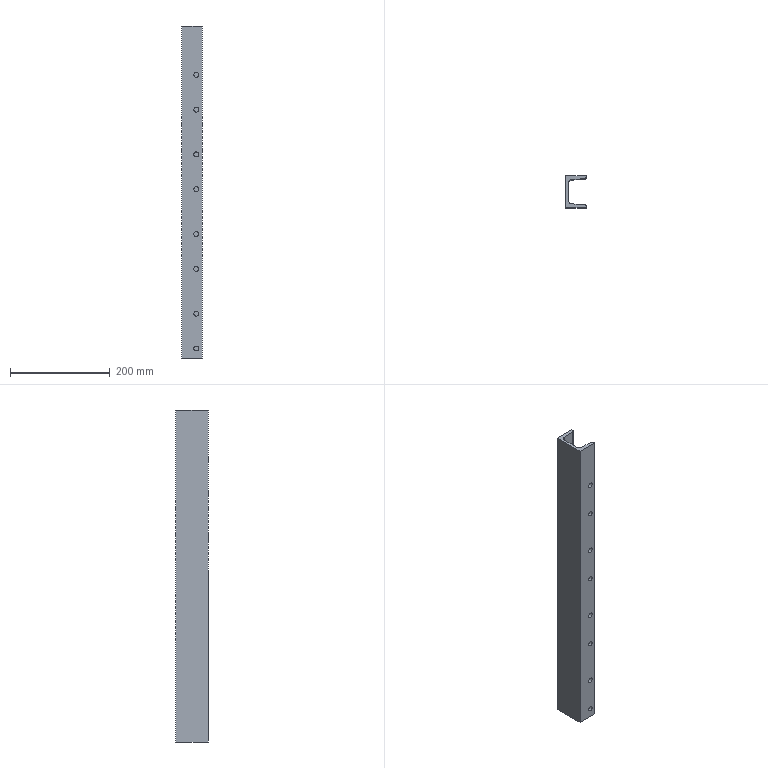Part | STEP file | DIN 1026-1 U 65 1785352380286 | 1 solid | 22 faces | box 42 x 65 x 667.157 mm | volume 598322 mm3 | cylinder 12 | plane 10 | commonest cylinder face diameters 10 x8 8 x2 15 x2
STEP:
#1=CARTESIAN_POINT('',(24.5,-32.5,449.081));
#2=VERTEX_POINT('',#1);
#3=CARTESIAN_POINT('',(29.5,-32.5,449.081));
#4=DIRECTION('',(0.,1.,0.));
#5=DIRECTION('',(1.,0.,0.));
#6=AXIS2_PLACEMENT_3D('',#3,#4,#5);
#7=CIRCLE('',#6,5.);
#8=EDGE_CURVE('',#2,#2,#7,.T.);
#9=ORIENTED_EDGE('',*,*,#8,.F.);
#10=CARTESIAN_POINT('',(24.5,-25.28,449.081));
#11=VERTEX_POINT('',#10);
#12=CARTESIAN_POINT('',(24.5,-32.5,449.081));
#13=DIRECTION('',(0.,1.,0.));
#14=VECTOR('',#13,5.);
#15=LINE('',#12,#14);
#16=EDGE_CURVE('',#2,#11,#15,.T.);
#17=ORIENTED_EDGE('',*,*,#16,.T.);
#18=CARTESIAN_POINT('',(29.5,-25.68,449.081));
#19=DIRECTION('',(-0.07975,-0.9968,0.));
#20=DIRECTION('',(0.9968,-0.07975,0.));
#21=AXIS2_PLACEMENT_3D('',#18,#19,#20);
#22=ELLIPSE('',#21,5.016,5.);
#23=EDGE_CURVE('',#11,#11,#22,.T.);
#24=ORIENTED_EDGE('',*,*,#23,.F.);
#25=ORIENTED_EDGE('',*,*,#16,.F.);
#26=EDGE_LOOP('',(#9,#17,#24,#25));
#27=FACE_OUTER_BOUND('',#26,.T.);
#28=CARTESIAN_POINT('',(29.5,-32.5,449.081));
#29=DIRECTION('',(0.,1.,0.));
#30=DIRECTION('',(1.,0.,0.));
#31=AXIS2_PLACEMENT_3D('',#28,#29,#30);
#32=CYLINDRICAL_SURFACE('',#31,5.);
#33=ADVANCED_FACE('',(#27),#32,.F.);
#34=CARTESIAN_POINT('',(24.5,-32.5,519.081));
#35=VERTEX_POINT('',#34);
#36=CARTESIAN_POINT('',(29.5,-32.5,519.081));
#37=DIRECTION('',(0.,1.,0.));
#38=DIRECTION('',(1.,0.,0.));
#39=AXIS2_PLACEMENT_3D('',#36,#37,#38);
#40=CIRCLE('',#39,5.);
#41=EDGE_CURVE('',#35,#35,#40,.T.);
#42=ORIENTED_EDGE('',*,*,#41,.F.);
#43=CARTESIAN_POINT('',(24.5,-25.28,519.081));
#44=VERTEX_POINT('',#43);
#45=CARTESIAN_POINT('',(24.5,-32.5,519.081));
#46=DIRECTION('',(0.,1.,0.));
#47=VECTOR('',#46,5.);
#48=LINE('',#45,#47);
#49=EDGE_CURVE('',#35,#44,#48,.T.);
#50=ORIENTED_EDGE('',*,*,#49,.T.);
#51=CARTESIAN_POINT('',(29.5,-25.68,519.081));
#52=DIRECTION('',(-0.07975,-0.9968,0.));
#53=DIRECTION('',(0.9968,-0.07975,0.));
#54=AXIS2_PLACEMENT_3D('',#51,#52,#53);
#55=ELLIPSE('',#54,5.016,5.);
#56=EDGE_CURVE('',#44,#44,#55,.T.);
#57=ORIENTED_EDGE('',*,*,#56,.F.);
#58=ORIENTED_EDGE('',*,*,#49,.F.);
#59=EDGE_LOOP('',(#42,#50,#57,#58));
#60=FACE_OUTER_BOUND('',#59,.T.);
#61=CARTESIAN_POINT('',(29.5,-32.5,519.081));
#62=DIRECTION('',(0.,1.,0.));
#63=DIRECTION('',(1.,0.,0.));
#64=AXIS2_PLACEMENT_3D('',#61,#62,#63);
#65=CYLINDRICAL_SURFACE('',#64,5.);
#66=ADVANCED_FACE('',(#60),#65,.F.);
#67=CARTESIAN_POINT('',(24.5,-32.5,289.081));
#68=VERTEX_POINT('',#67);
#69=CARTESIAN_POINT('',(29.5,-32.5,289.081));
#70=DIRECTION('',(0.,1.,0.));
#71=DIRECTION('',(1.,0.,0.));
#72=AXIS2_PLACEMENT_3D('',#69,#70,#71);
#73=CIRCLE('',#72,5.);
#74=EDGE_CURVE('',#68,#68,#73,.T.);
#75=ORIENTED_EDGE('',*,*,#74,.F.);
#76=CARTESIAN_POINT('',(24.5,-25.28,289.081));
#77=VERTEX_POINT('',#76);
#78=CARTESIAN_POINT('',(24.5,-32.5,289.081));
#79=DIRECTION('',(0.,1.,0.));
#80=VECTOR('',#79,5.);
#81=LINE('',#78,#80);
#82=EDGE_CURVE('',#68,#77,#81,.T.);
#83=ORIENTED_EDGE('',*,*,#82,.T.);
#84=CARTESIAN_POINT('',(29.5,-25.68,289.081));
#85=DIRECTION('',(-0.07975,-0.9968,0.));
#86=DIRECTION('',(0.9968,-0.07975,0.));
#87=AXIS2_PLACEMENT_3D('',#84,#85,#86);
#88=ELLIPSE('',#87,5.016,5.);
#89=EDGE_CURVE('',#77,#77,#88,.T.);
#90=ORIENTED_EDGE('',*,*,#89,.F.);
#91=ORIENTED_EDGE('',*,*,#82,.F.);
#92=EDGE_LOOP('',(#75,#83,#90,#91));
#93=FACE_OUTER_BOUND('',#92,.T.);
#94=CARTESIAN_POINT('',(29.5,-32.5,289.081));
#95=DIRECTION('',(0.,1.,0.));
#96=DIRECTION('',(1.,0.,0.));
#97=AXIS2_PLACEMENT_3D('',#94,#95,#96);
#98=CYLINDRICAL_SURFACE('',#97,5.);
#99=ADVANCED_FACE('',(#93),#98,.F.);
#100=CARTESIAN_POINT('',(24.5,-32.5,359.081));
#101=VERTEX_POINT('',#100);
#102=CARTESIAN_POINT('',(29.5,-32.5,359.081));
#103=DIRECTION('',(0.,1.,0.));
#104=DIRECTION('',(1.,0.,0.));
#105=AXIS2_PLACEMENT_3D('',#102,#103,#104);
#106=CIRCLE('',#105,5.);
#107=EDGE_CURVE('',#101,#101,#106,.T.);
#108=ORIENTED_EDGE('',*,*,#107,.F.);
#109=CARTESIAN_POINT('',(24.5,-25.28,359.081));
#110=VERTEX_POINT('',#109);
#111=CARTESIAN_POINT('',(24.5,-32.5,359.081));
#112=DIRECTION('',(0.,1.,0.));
#113=VECTOR('',#112,5.);
#114=LINE('',#111,#113);
#115=EDGE_CURVE('',#101,#110,#114,.T.);
#116=ORIENTED_EDGE('',*,*,#115,.T.);
#117=CARTESIAN_POINT('',(29.5,-25.68,359.081));
#118=DIRECTION('',(-0.07975,-0.9968,0.));
#119=DIRECTION('',(0.9968,-0.07975,0.));
#120=AXIS2_PLACEMENT_3D('',#117,#118,#119);
#121=ELLIPSE('',#120,5.016,5.);
#122=EDGE_CURVE('',#110,#110,#121,.T.);
#123=ORIENTED_EDGE('',*,*,#122,.F.);
#124=ORIENTED_EDGE('',*,*,#115,.F.);
#125=EDGE_LOOP('',(#108,#116,#123,#124));
#126=FACE_OUTER_BOUND('',#125,.T.);
#127=CARTESIAN_POINT('',(29.5,-32.5,359.081));
#128=DIRECTION('',(0.,1.,0.));
#129=DIRECTION('',(1.,0.,0.));
#130=AXIS2_PLACEMENT_3D('',#127,#128,#129);
#131=CYLINDRICAL_SURFACE('',#130,5.);
#132=ADVANCED_FACE('',(#126),#131,.F.);
#133=CARTESIAN_POINT('',(24.5,-32.5,129.081));
#134=VERTEX_POINT('',#133);
#135=CARTESIAN_POINT('',(29.5,-32.5,129.081));
#136=DIRECTION('',(0.,1.,0.));
#137=DIRECTION('',(1.,0.,0.));
#138=AXIS2_PLACEMENT_3D('',#135,#136,#137);
#139=CIRCLE('',#138,5.);
#140=EDGE_CURVE('',#134,#134,#139,.T.);
#141=ORIENTED_EDGE('',*,*,#140,.F.);
#142=CARTESIAN_POINT('',(24.5,-25.28,129.081));
#143=VERTEX_POINT('',#142);
#144=CARTESIAN_POINT('',(24.5,-32.5,129.081));
#145=DIRECTION('',(0.,1.,0.));
#146=VECTOR('',#145,5.);
#147=LINE('',#144,#146);
#148=EDGE_CURVE('',#134,#143,#147,.T.);
#149=ORIENTED_EDGE('',*,*,#148,.T.);
#150=CARTESIAN_POINT('',(29.5,-25.68,129.081));
#151=DIRECTION('',(-0.07975,-0.9968,0.));
#152=DIRECTION('',(0.9968,-0.07975,0.));
#153=AXIS2_PLACEMENT_3D('',#150,#151,#152);
#154=ELLIPSE('',#153,5.016,5.);
#155=EDGE_CURVE('',#143,#143,#154,.T.);
#156=ORIENTED_EDGE('',*,*,#155,.F.);
#157=ORIENTED_EDGE('',*,*,#148,.F.);
#158=EDGE_LOOP('',(#141,#149,#156,#157));
#159=FACE_OUTER_BOUND('',#158,.T.);
#160=CARTESIAN_POINT('',(29.5,-32.5,129.081));
#161=DIRECTION('',(0.,1.,0.));
#162=DIRECTION('',(1.,0.,0.));
#163=AXIS2_PLACEMENT_3D('',#160,#161,#162);
#164=CYLINDRICAL_SURFACE('',#163,5.);
#165=ADVANCED_FACE('',(#159),#164,.F.);
#166=CARTESIAN_POINT('',(24.5,-32.5,199.081));
#167=VERTEX_POINT('',#166);
#168=CARTESIAN_POINT('',(29.5,-32.5,199.081));
#169=DIRECTION('',(0.,1.,0.));
#170=DIRECTION('',(1.,0.,0.));
#171=AXIS2_PLACEMENT_3D('',#168,#169,#170);
#172=CIRCLE('',#171,5.);
#173=EDGE_CURVE('',#167,#167,#172,.T.);
#174=ORIENTED_EDGE('',*,*,#173,.F.);
#175=CARTESIAN_POINT('',(24.5,-25.28,199.081));
#176=VERTEX_POINT('',#175);
#177=CARTESIAN_POINT('',(24.5,-32.5,199.081));
#178=DIRECTION('',(0.,1.,0.));
#179=VECTOR('',#178,5.);
#180=LINE('',#177,#179);
#181=EDGE_CURVE('',#167,#176,#180,.T.);
#182=ORIENTED_EDGE('',*,*,#181,.T.);
#183=CARTESIAN_POINT('',(29.5,-25.68,199.081));
#184=DIRECTION('',(-0.07975,-0.9968,0.));
#185=DIRECTION('',(0.9968,-0.07975,0.));
#186=AXIS2_PLACEMENT_3D('',#183,#184,#185);
#187=ELLIPSE('',#186,5.016,5.);
#188=EDGE_CURVE('',#176,#176,#187,.T.);
#189=ORIENTED_EDGE('',*,*,#188,.F.);
#190=ORIENTED_EDGE('',*,*,#181,.F.);
#191=EDGE_LOOP('',(#174,#182,#189,#190));
#192=FACE_OUTER_BOUND('',#191,.T.);
#193=CARTESIAN_POINT('',(29.5,-32.5,199.081));
#194=DIRECTION('',(0.,1.,0.));
#195=DIRECTION('',(1.,0.,0.));
#196=AXIS2_PLACEMENT_3D('',#193,#194,#195);
#197=CYLINDRICAL_SURFACE('',#196,5.);
#198=ADVANCED_FACE('',(#192),#197,.F.);
#199=CARTESIAN_POINT('',(24.5,-32.5,-30.919));
#200=VERTEX_POINT('',#199);
#201=CARTESIAN_POINT('',(29.5,-32.5,-30.919));
#202=DIRECTION('',(0.,1.,0.));
#203=DIRECTION('',(1.,0.,0.));
#204=AXIS2_PLACEMENT_3D('',#201,#202,#203);
#205=CIRCLE('',#204,5.);
#206=EDGE_CURVE('',#200,#200,#205,.T.);
#207=ORIENTED_EDGE('',*,*,#206,.F.);
#208=CARTESIAN_POINT('',(24.5,-25.28,-30.919));
#209=VERTEX_POINT('',#208);
#210=CARTESIAN_POINT('',(24.5,-32.5,-30.919));
#211=DIRECTION('',(0.,1.,0.));
#212=VECTOR('',#211,5.);
#213=LINE('',#210,#212);
#214=EDGE_CURVE('',#200,#209,#213,.T.);
#215=ORIENTED_EDGE('',*,*,#214,.T.);
#216=CARTESIAN_POINT('',(29.5,-25.68,-30.919));
#217=DIRECTION('',(-0.07975,-0.9968,0.));
#218=DIRECTION('',(0.9968,-0.07975,0.));
#219=AXIS2_PLACEMENT_3D('',#216,#217,#218);
#220=ELLIPSE('',#219,5.016,5.);
#221=EDGE_CURVE('',#209,#209,#220,.T.);
#222=ORIENTED_EDGE('',*,*,#221,.F.);
#223=ORIENTED_EDGE('',*,*,#214,.F.);
#224=EDGE_LOOP('',(#207,#215,#222,#223));
#225=FACE_OUTER_BOUND('',#224,.T.);
#226=CARTESIAN_POINT('',(29.5,-32.5,-30.919));
#227=DIRECTION('',(0.,1.,0.));
#228=DIRECTION('',(1.,0.,0.));
#229=AXIS2_PLACEMENT_3D('',#226,#227,#228);
#230=CYLINDRICAL_SURFACE('',#229,5.);
#231=ADVANCED_FACE('',(#225),#230,.F.);
#232=CARTESIAN_POINT('',(24.5,-32.5,39.081));
#233=VERTEX_POINT('',#232);
#234=CARTESIAN_POINT('',(29.5,-32.5,39.081));
#235=DIRECTION('',(0.,1.,0.));
#236=DIRECTION('',(1.,0.,0.));
#237=AXIS2_PLACEMENT_3D('',#234,#235,#236);
#238=CIRCLE('',#237,5.);
#239=EDGE_CURVE('',#233,#233,#238,.T.);
#240=ORIENTED_EDGE('',*,*,#239,.F.);
#241=CARTESIAN_POINT('',(24.5,-25.28,39.081));
#242=VERTEX_POINT('',#241);
#243=CARTESIAN_POINT('',(24.5,-32.5,39.081));
#244=DIRECTION('',(0.,1.,0.));
#245=VECTOR('',#244,5.);
#246=LINE('',#243,#245);
#247=EDGE_CURVE('',#233,#242,#246,.T.);
#248=ORIENTED_EDGE('',*,*,#247,.T.);
#249=CARTESIAN_POINT('',(29.5,-25.68,39.081));
#250=DIRECTION('',(-0.07975,-0.9968,0.));
#251=DIRECTION('',(0.9968,-0.07975,0.));
#252=AXIS2_PLACEMENT_3D('',#249,#250,#251);
#253=ELLIPSE('',#252,5.016,5.);
#254=EDGE_CURVE('',#242,#242,#253,.T.);
#255=ORIENTED_EDGE('',*,*,#254,.F.);
#256=ORIENTED_EDGE('',*,*,#247,.F.);
#257=EDGE_LOOP('',(#240,#248,#255,#256));
#258=FACE_OUTER_BOUND('',#257,.T.);
#259=CARTESIAN_POINT('',(29.5,-32.5,39.081));
#260=DIRECTION('',(0.,1.,0.));
#261=DIRECTION('',(1.,0.,0.));
#262=AXIS2_PLACEMENT_3D('',#259,#260,#261);
#263=CYLINDRICAL_SURFACE('',#262,5.);
#264=ADVANCED_FACE('',(#258),#263,.F.);
#265=CARTESIAN_POINT('',(5.5,-16.836,617.157));
#266=VERTEX_POINT('',#265);
#267=CARTESIAN_POINT('',(12.402,-24.312,617.157));
#268=VERTEX_POINT('',#267);
#269=CARTESIAN_POINT('',(13.,-16.836,617.157));
#270=DIRECTION('',(0.,0.,1.));
#271=DIRECTION('',(-1.,0.,0.));
#272=AXIS2_PLACEMENT_3D('',#269,#270,#271);
#273=CIRCLE('',#272,7.5);
#274=EDGE_CURVE('',#266,#268,#273,.T.);
#275=ORIENTED_EDGE('',*,*,#274,.T.);
#276=CARTESIAN_POINT('',(12.402,-24.312,-50.));
#277=VERTEX_POINT('',#276);
#278=CARTESIAN_POINT('',(12.402,-24.312,0.));
#279=DIRECTION('',(0.,0.,-1.));
#280=VECTOR('',#279,10.);
#281=LINE('',#278,#280);
#282=EDGE_CURVE('',#268,#277,#281,.T.);
#283=ORIENTED_EDGE('',*,*,#282,.T.);
#284=CARTESIAN_POINT('',(5.5,-16.836,-50.));
#285=VERTEX_POINT('',#284);
#286=CARTESIAN_POINT('',(13.,-16.836,-50.));
#287=DIRECTION('',(0.,0.,1.));
#288=DIRECTION('',(-1.,0.,0.));
#289=AXIS2_PLACEMENT_3D('',#286,#287,#288);
#290=CIRCLE('',#289,7.5);
#291=EDGE_CURVE('',#285,#277,#290,.T.);
#292=ORIENTED_EDGE('',*,*,#291,.F.);
#293=CARTESIAN_POINT('',(5.5,-16.836,0.));
#294=DIRECTION('',(0.,0.,-1.));
#295=VECTOR('',#294,10.);
#296=LINE('',#293,#295);
#297=EDGE_CURVE('',#266,#285,#296,.T.);
#298=ORIENTED_EDGE('',*,*,#297,.F.);
#299=EDGE_LOOP('',(#275,#283,#292,#298));
#300=FACE_OUTER_BOUND('',#299,.T.);
#301=CARTESIAN_POINT('',(13.,-16.836,0.));
#302=DIRECTION('',(0.,0.,1.));
#303=DIRECTION('',(-1.,0.,0.));
#304=AXIS2_PLACEMENT_3D('',#301,#302,#303);
#305=CYLINDRICAL_SURFACE('',#304,7.5);
#306=ADVANCED_FACE('',(#300),#305,.F.);
#307=CARTESIAN_POINT('',(38.319,-26.386,617.157));
#308=VERTEX_POINT('',#307);
#309=CARTESIAN_POINT('',(15.707,-24.577,617.157));
#310=DIRECTION('',(0.9968,-0.07975,0.));
#311=VECTOR('',#310,10.);
#312=LINE('',#309,#311);
#313=EDGE_CURVE('',#268,#308,#312,.T.);
#314=ORIENTED_EDGE('',*,*,#313,.T.);
#315=CARTESIAN_POINT('',(38.319,-26.386,-50.));
#316=VERTEX_POINT('',#315);
#317=CARTESIAN_POINT('',(38.319,-26.386,0.));
#318=DIRECTION('',(0.,0.,-1.));
#319=VECTOR('',#318,10.);
#320=LINE('',#317,#319);
#321=EDGE_CURVE('',#308,#316,#320,.T.);
#322=ORIENTED_EDGE('',*,*,#321,.T.);
#323=CARTESIAN_POINT('',(15.707,-24.577,-50.));
#324=DIRECTION('',(0.9968,-0.07975,0.));
#325=VECTOR('',#324,10.);
#326=LINE('',#323,#325);
#327=EDGE_CURVE('',#277,#316,#326,.T.);
#328=ORIENTED_EDGE('',*,*,#327,.F.);
#329=ORIENTED_EDGE('',*,*,#282,.F.);
#330=EDGE_LOOP('',(#314,#322,#328,#329));
#331=FACE_OUTER_BOUND('',#330,.T.);
#332=ORIENTED_EDGE('',*,*,#23,.T.);
#333=EDGE_LOOP('',(#332));
#334=FACE_BOUND('',#333,.T.);
#335=ORIENTED_EDGE('',*,*,#56,.T.);
#336=EDGE_LOOP('',(#335));
#337=FACE_BOUND('',#336,.T.);
#338=ORIENTED_EDGE('',*,*,#89,.T.);
#339=EDGE_LOOP('',(#338));
#340=FACE_BOUND('',#339,.T.);
#341=ORIENTED_EDGE('',*,*,#122,.T.);
#342=EDGE_LOOP('',(#341));
#343=FACE_BOUND('',#342,.T.);
#344=ORIENTED_EDGE('',*,*,#155,.T.);
#345=EDGE_LOOP('',(#344));
#346=FACE_BOUND('',#345,.T.);
#347=ORIENTED_EDGE('',*,*,#188,.T.);
#348=EDGE_LOOP('',(#347));
#349=FACE_BOUND('',#348,.T.);
#350=ORIENTED_EDGE('',*,*,#221,.T.);
#351=EDGE_LOOP('',(#350));
#352=FACE_BOUND('',#351,.T.);
#353=ORIENTED_EDGE('',*,*,#254,.T.);
#354=EDGE_LOOP('',(#353));
#355=FACE_BOUND('',#354,.T.);
#356=CARTESIAN_POINT('',(12.402,-24.312,0.));
#357=DIRECTION('',(0.07975,0.9968,0.));
#358=DIRECTION('',(0.,0.,1.));
#359=AXIS2_PLACEMENT_3D('',#356,#357,#358);
#360=PLANE('',#359);
#361=ADVANCED_FACE('',(#331,#334,#337,#340,#343,#346,#349,#352,#355),#360,.T.);
#362=CARTESIAN_POINT('',(42.,-30.373,617.157));
#363=VERTEX_POINT('',#362);
#364=CARTESIAN_POINT('',(38.,-30.373,617.157));
#365=DIRECTION('',(0.,0.,-1.));
#366=DIRECTION('',(-1.,0.,0.));
#367=AXIS2_PLACEMENT_3D('',#364,#365,#366);
#368=CIRCLE('',#367,4.);
#369=EDGE_CURVE('',#308,#363,#368,.T.);
#370=ORIENTED_EDGE('',*,*,#369,.T.);
#371=CARTESIAN_POINT('',(42.,-30.373,-50.));
#372=VERTEX_POINT('',#371);
#373=CARTESIAN_POINT('',(42.,-30.373,0.));
#374=DIRECTION('',(0.,0.,-1.));
#375=VECTOR('',#374,10.);
#376=LINE('',#373,#375);
#377=EDGE_CURVE('',#363,#372,#376,.T.);
#378=ORIENTED_EDGE('',*,*,#377,.T.);
#379=CARTESIAN_POINT('',(38.,-30.373,-50.));
#380=DIRECTION('',(0.,0.,-1.));
#381=DIRECTION('',(-1.,0.,0.));
#382=AXIS2_PLACEMENT_3D('',#379,#380,#381);
#383=CIRCLE('',#382,4.);
#384=EDGE_CURVE('',#316,#372,#383,.T.);
#385=ORIENTED_EDGE('',*,*,#384,.F.);
#386=ORIENTED_EDGE('',*,*,#321,.F.);
#387=EDGE_LOOP('',(#370,#378,#385,#386));
#388=FACE_OUTER_BOUND('',#387,.T.);
#389=CARTESIAN_POINT('',(38.,-30.373,0.));
#390=DIRECTION('',(0.,0.,1.));
#391=DIRECTION('',(-1.,0.,0.));
#392=AXIS2_PLACEMENT_3D('',#389,#390,#391);
#393=CYLINDRICAL_SURFACE('',#392,4.);
#394=ADVANCED_FACE('',(#388),#393,.T.);
#395=CARTESIAN_POINT('',(42.,-32.5,617.157));
#396=VERTEX_POINT('',#395);
#397=CARTESIAN_POINT('',(42.,-15.186,617.157));
#398=DIRECTION('',(0.,-1.,0.));
#399=VECTOR('',#398,10.);
#400=LINE('',#397,#399);
#401=EDGE_CURVE('',#363,#396,#400,.T.);
#402=ORIENTED_EDGE('',*,*,#401,.T.);
#403=CARTESIAN_POINT('',(42.,-32.5,-50.));
#404=VERTEX_POINT('',#403);
#405=CARTESIAN_POINT('',(42.,-32.5,0.));
#406=DIRECTION('',(0.,0.,-1.));
#407=VECTOR('',#406,10.);
#408=LINE('',#405,#407);
#409=EDGE_CURVE('',#396,#404,#408,.T.);
#410=ORIENTED_EDGE('',*,*,#409,.T.);
#411=CARTESIAN_POINT('',(42.,-15.186,-50.));
#412=DIRECTION('',(0.,-1.,0.));
#413=VECTOR('',#412,10.);
#414=LINE('',#411,#413);
#415=EDGE_CURVE('',#372,#404,#414,.T.);
#416=ORIENTED_EDGE('',*,*,#415,.F.);
#417=ORIENTED_EDGE('',*,*,#377,.F.);
#418=EDGE_LOOP('',(#402,#410,#416,#417));
#419=FACE_OUTER_BOUND('',#418,.T.);
#420=CARTESIAN_POINT('',(42.,-30.373,0.));
#421=DIRECTION('',(1.,0.,0.));
#422=DIRECTION('',(0.,0.,-1.));
#423=AXIS2_PLACEMENT_3D('',#420,#421,#422);
#424=PLANE('',#423);
#425=ADVANCED_FACE('',(#419),#424,.T.);
#426=CARTESIAN_POINT('',(0.,-32.5,617.157));
#427=VERTEX_POINT('',#426);
#428=CARTESIAN_POINT('',(31.5,-32.5,617.157));
#429=DIRECTION('',(-1.,0.,0.));
#430=VECTOR('',#429,10.);
#431=LINE('',#428,#430);
#432=EDGE_CURVE('',#396,#427,#431,.T.);
#433=ORIENTED_EDGE('',*,*,#432,.T.);
#434=CARTESIAN_POINT('',(0.,-32.5,-50.));
#435=VERTEX_POINT('',#434);
#436=CARTESIAN_POINT('',(0.,-32.5,0.));
#437=DIRECTION('',(0.,0.,-1.));
#438=VECTOR('',#437,10.);
#439=LINE('',#436,#438);
#440=EDGE_CURVE('',#427,#435,#439,.T.);
#441=ORIENTED_EDGE('',*,*,#440,.T.);
#442=CARTESIAN_POINT('',(31.5,-32.5,-50.));
#443=DIRECTION('',(-1.,0.,0.));
#444=VECTOR('',#443,10.);
#445=LINE('',#442,#444);
#446=EDGE_CURVE('',#404,#435,#445,.T.);
#447=ORIENTED_EDGE('',*,*,#446,.F.);
#448=ORIENTED_EDGE('',*,*,#409,.F.);
#449=EDGE_LOOP('',(#433,#441,#447,#448));
#450=FACE_OUTER_BOUND('',#449,.T.);
#451=ORIENTED_EDGE('',*,*,#8,.T.);
#452=EDGE_LOOP('',(#451));
#453=FACE_BOUND('',#452,.T.);
#454=ORIENTED_EDGE('',*,*,#41,.T.);
#455=EDGE_LOOP('',(#454));
#456=FACE_BOUND('',#455,.T.);
#457=ORIENTED_EDGE('',*,*,#74,.T.);
#458=EDGE_LOOP('',(#457));
#459=FACE_BOUND('',#458,.T.);
#460=ORIENTED_EDGE('',*,*,#107,.T.);
#461=EDGE_LOOP('',(#460));
#462=FACE_BOUND('',#461,.T.);
#463=ORIENTED_EDGE('',*,*,#140,.T.);
#464=EDGE_LOOP('',(#463));
#465=FACE_BOUND('',#464,.T.);
#466=ORIENTED_EDGE('',*,*,#173,.T.);
#467=EDGE_LOOP('',(#466));
#468=FACE_BOUND('',#467,.T.);
#469=ORIENTED_EDGE('',*,*,#206,.T.);
#470=EDGE_LOOP('',(#469));
#471=FACE_BOUND('',#470,.T.);
#472=ORIENTED_EDGE('',*,*,#239,.T.);
#473=EDGE_LOOP('',(#472));
#474=FACE_BOUND('',#473,.T.);
#475=CARTESIAN_POINT('',(42.,-32.5,0.));
#476=DIRECTION('',(0.,-1.,0.));
#477=DIRECTION('',(0.,0.,-1.));
#478=AXIS2_PLACEMENT_3D('',#475,#476,#477);
#479=PLANE('',#478);
#480=ADVANCED_FACE('',(#450,#453,#456,#459,#462,#465,#468,#471,#474),#479,.T.);
#481=CARTESIAN_POINT('',(0.,32.5,617.157));
#482=VERTEX_POINT('',#481);
#483=CARTESIAN_POINT('',(0.,0.,617.157));
#484=DIRECTION('',(0.,1.,0.));
#485=VECTOR('',#484,10.);
#486=LINE('',#483,#485);
#487=EDGE_CURVE('',#427,#482,#486,.T.);
#488=ORIENTED_EDGE('',*,*,#487,.T.);
#489=CARTESIAN_POINT('',(0.,32.5,-50.));
#490=VERTEX_POINT('',#489);
#491=CARTESIAN_POINT('',(0.,32.5,0.));
#492=DIRECTION('',(0.,0.,-1.));
#493=VECTOR('',#492,10.);
#494=LINE('',#491,#493);
#495=EDGE_CURVE('',#482,#490,#494,.T.);
#496=ORIENTED_EDGE('',*,*,#495,.T.);
#497=CARTESIAN_POINT('',(0.,0.,-50.));
#498=DIRECTION('',(0.,1.,0.));
#499=VECTOR('',#498,10.);
#500=LINE('',#497,#499);
#501=EDGE_CURVE('',#435,#490,#500,.T.);
#502=ORIENTED_EDGE('',*,*,#501,.F.);
#503=ORIENTED_EDGE('',*,*,#440,.F.);
#504=EDGE_LOOP('',(#488,#496,#502,#503));
#505=FACE_OUTER_BOUND('',#504,.T.);
#506=CARTESIAN_POINT('',(0.,0.,0.));
#507=DIRECTION('',(-1.,0.,0.));
#508=DIRECTION('',(0.,0.,1.));
#509=AXIS2_PLACEMENT_3D('',#506,#507,#508);
#510=PLANE('',#509);
#511=ADVANCED_FACE('',(#505),#510,.T.);
#512=CARTESIAN_POINT('',(42.,32.5,617.157));
#513=VERTEX_POINT('',#512);
#514=CARTESIAN_POINT('',(10.5,32.5,617.157));
#515=DIRECTION('',(1.,0.,0.));
#516=VECTOR('',#515,10.);
#517=LINE('',#514,#516);
#518=EDGE_CURVE('',#482,#513,#517,.T.);
#519=ORIENTED_EDGE('',*,*,#518,.T.);
#520=CARTESIAN_POINT('',(42.,32.5,-50.));
#521=VERTEX_POINT('',#520);
#522=CARTESIAN_POINT('',(42.,32.5,0.));
#523=DIRECTION('',(0.,0.,-1.));
#524=VECTOR('',#523,10.);
#525=LINE('',#522,#524);
#526=EDGE_CURVE('',#513,#521,#525,.T.);
#527=ORIENTED_EDGE('',*,*,#526,.T.);
#528=CARTESIAN_POINT('',(10.5,32.5,-50.));
#529=DIRECTION('',(1.,0.,0.));
#530=VECTOR('',#529,10.);
#531=LINE('',#528,#530);
#532=EDGE_CURVE('',#490,#521,#531,.T.);
#533=ORIENTED_EDGE('',*,*,#532,.F.);
#534=ORIENTED_EDGE('',*,*,#495,.F.);
#535=EDGE_LOOP('',(#519,#527,#533,#534));
#536=FACE_OUTER_BOUND('',#535,.T.);
#537=CARTESIAN_POINT('',(0.,32.5,0.));
#538=DIRECTION('',(0.,1.,0.));
#539=DIRECTION('',(0.,0.,1.));
#540=AXIS2_PLACEMENT_3D('',#537,#538,#539);
#541=PLANE('',#540);
#542=ADVANCED_FACE('',(#536),#541,.T.);
#543=CARTESIAN_POINT('',(42.,30.373,617.157));
#544=VERTEX_POINT('',#543);
#545=CARTESIAN_POINT('',(42.,16.25,617.157));
#546=DIRECTION('',(0.,-1.,0.));
#547=VECTOR('',#546,10.);
#548=LINE('',#545,#547);
#549=EDGE_CURVE('',#513,#544,#548,.T.);
#550=ORIENTED_EDGE('',*,*,#549,.T.);
#551=CARTESIAN_POINT('',(42.,30.373,-50.));
#552=VERTEX_POINT('',#551);
#553=CARTESIAN_POINT('',(42.,30.373,0.));
#554=DIRECTION('',(0.,0.,-1.));
#555=VECTOR('',#554,10.);
#556=LINE('',#553,#555);
#557=EDGE_CURVE('',#544,#552,#556,.T.);
#558=ORIENTED_EDGE('',*,*,#557,.T.);
#559=CARTESIAN_POINT('',(42.,16.25,-50.));
#560=DIRECTION('',(0.,-1.,0.));
#561=VECTOR('',#560,10.);
#562=LINE('',#559,#561);
#563=EDGE_CURVE('',#521,#552,#562,.T.);
#564=ORIENTED_EDGE('',*,*,#563,.F.);
#565=ORIENTED_EDGE('',*,*,#526,.F.);
#566=EDGE_LOOP('',(#550,#558,#564,#565));
#567=FACE_OUTER_BOUND('',#566,.T.);
#568=CARTESIAN_POINT('',(42.,32.5,0.));
#569=DIRECTION('',(1.,0.,0.));
#570=DIRECTION('',(0.,0.,-1.));
#571=AXIS2_PLACEMENT_3D('',#568,#569,#570);
#572=PLANE('',#571);
#573=ADVANCED_FACE('',(#567),#572,.T.);
#574=CARTESIAN_POINT('',(38.319,26.386,617.157));
#575=VERTEX_POINT('',#574);
#576=CARTESIAN_POINT('',(38.,30.373,617.157));
#577=DIRECTION('',(0.,0.,-1.));
#578=DIRECTION('',(-0.07975,0.9968,0.));
#579=AXIS2_PLACEMENT_3D('',#576,#577,#578);
#580=CIRCLE('',#579,4.);
#581=EDGE_CURVE('',#544,#575,#580,.T.);
#582=ORIENTED_EDGE('',*,*,#581,.T.);
#583=CARTESIAN_POINT('',(38.319,26.386,-50.));
#584=VERTEX_POINT('',#583);
#585=CARTESIAN_POINT('',(38.319,26.386,0.));
#586=DIRECTION('',(0.,0.,-1.));
#587=VECTOR('',#586,10.);
#588=LINE('',#585,#587);
#589=EDGE_CURVE('',#575,#584,#588,.T.);
#590=ORIENTED_EDGE('',*,*,#589,.T.);
#591=CARTESIAN_POINT('',(38.,30.373,-50.));
#592=DIRECTION('',(0.,0.,-1.));
#593=DIRECTION('',(-0.07975,0.9968,0.));
#594=AXIS2_PLACEMENT_3D('',#591,#592,#593);
#595=CIRCLE('',#594,4.);
#596=EDGE_CURVE('',#552,#584,#595,.T.);
#597=ORIENTED_EDGE('',*,*,#596,.F.);
#598=ORIENTED_EDGE('',*,*,#557,.F.);
#599=EDGE_LOOP('',(#582,#590,#597,#598));
#600=FACE_OUTER_BOUND('',#599,.T.);
#601=CARTESIAN_POINT('',(38.,30.373,0.));
#602=DIRECTION('',(0.,0.,1.));
#603=DIRECTION('',(-0.07975,0.9968,0.));
#604=AXIS2_PLACEMENT_3D('',#601,#602,#603);
#605=CYLINDRICAL_SURFACE('',#604,4.);
#606=ADVANCED_FACE('',(#600),#605,.T.);
#607=CARTESIAN_POINT('',(12.402,24.312,617.157));
#608=VERTEX_POINT('',#607);
#609=CARTESIAN_POINT('',(28.666,25.613,617.157));
#610=DIRECTION('',(-0.9968,-0.07975,0.));
#611=VECTOR('',#610,10.);
#612=LINE('',#609,#611);
#613=EDGE_CURVE('',#575,#608,#612,.T.);
#614=ORIENTED_EDGE('',*,*,#613,.T.);
#615=CARTESIAN_POINT('',(12.402,24.312,-50.));
#616=VERTEX_POINT('',#615);
#617=CARTESIAN_POINT('',(12.402,24.312,0.));
#618=DIRECTION('',(0.,0.,-1.));
#619=VECTOR('',#618,10.);
#620=LINE('',#617,#619);
#621=EDGE_CURVE('',#608,#616,#620,.T.);
#622=ORIENTED_EDGE('',*,*,#621,.T.);
#623=CARTESIAN_POINT('',(28.666,25.613,-50.));
#624=DIRECTION('',(-0.9968,-0.07975,0.));
#625=VECTOR('',#624,10.);
#626=LINE('',#623,#625);
#627=EDGE_CURVE('',#584,#616,#626,.T.);
#628=ORIENTED_EDGE('',*,*,#627,.F.);
#629=ORIENTED_EDGE('',*,*,#589,.F.);
#630=EDGE_LOOP('',(#614,#622,#628,#629));
#631=FACE_OUTER_BOUND('',#630,.T.);
#632=CARTESIAN_POINT('',(38.319,26.386,0.));
#633=DIRECTION('',(0.07975,-0.9968,0.));
#634=DIRECTION('',(0.,0.,-1.));
#635=AXIS2_PLACEMENT_3D('',#632,#633,#634);
#636=PLANE('',#635);
#637=ADVANCED_FACE('',(#631),#636,.T.);
#638=CARTESIAN_POINT('',(5.5,16.836,617.157));
#639=VERTEX_POINT('',#638);
#640=CARTESIAN_POINT('',(13.,16.836,617.157));
#641=DIRECTION('',(0.,0.,1.));
#642=DIRECTION('',(-0.07975,0.9968,0.));
#643=AXIS2_PLACEMENT_3D('',#640,#641,#642);
#644=CIRCLE('',#643,7.5);
#645=EDGE_CURVE('',#608,#639,#644,.T.);
#646=ORIENTED_EDGE('',*,*,#645,.T.);
#647=CARTESIAN_POINT('',(5.5,16.836,-50.));
#648=VERTEX_POINT('',#647);
#649=CARTESIAN_POINT('',(5.5,16.836,0.));
#650=DIRECTION('',(0.,0.,-1.));
#651=VECTOR('',#650,10.);
#652=LINE('',#649,#651);
#653=EDGE_CURVE('',#639,#648,#652,.T.);
#654=ORIENTED_EDGE('',*,*,#653,.T.);
#655=CARTESIAN_POINT('',(13.,16.836,-50.));
#656=DIRECTION('',(0.,0.,1.));
#657=DIRECTION('',(-0.07975,0.9968,0.));
#658=AXIS2_PLACEMENT_3D('',#655,#656,#657);
#659=CIRCLE('',#658,7.5);
#660=EDGE_CURVE('',#616,#648,#659,.T.);
#661=ORIENTED_EDGE('',*,*,#660,.F.);
#662=ORIENTED_EDGE('',*,*,#621,.F.);
#663=EDGE_LOOP('',(#646,#654,#661,#662));
#664=FACE_OUTER_BOUND('',#663,.T.);
#665=CARTESIAN_POINT('',(13.,16.836,0.));
#666=DIRECTION('',(0.,0.,1.));
#667=DIRECTION('',(-0.07975,0.9968,0.));
#668=AXIS2_PLACEMENT_3D('',#665,#666,#667);
#669=CYLINDRICAL_SURFACE('',#668,7.5);
#670=ADVANCED_FACE('',(#664),#669,.F.);
#671=CARTESIAN_POINT('',(5.5,0.,617.157));
#672=DIRECTION('',(0.,-1.,0.));
#673=VECTOR('',#672,10.);
#674=LINE('',#671,#673);
#675=EDGE_CURVE('',#639,#266,#674,.T.);
#676=ORIENTED_EDGE('',*,*,#675,.T.);
#677=ORIENTED_EDGE('',*,*,#297,.T.);
#678=CARTESIAN_POINT('',(5.5,0.,-50.));
#679=DIRECTION('',(0.,-1.,0.));
#680=VECTOR('',#679,10.);
#681=LINE('',#678,#680);
#682=EDGE_CURVE('',#648,#285,#681,.T.);
#683=ORIENTED_EDGE('',*,*,#682,.F.);
#684=ORIENTED_EDGE('',*,*,#653,.F.);
#685=EDGE_LOOP('',(#676,#677,#683,#684));
#686=FACE_OUTER_BOUND('',#685,.T.);
#687=CARTESIAN_POINT('',(5.5,0.,0.));
#688=DIRECTION('',(1.,0.,0.));
#689=DIRECTION('',(0.,0.,-1.));
#690=AXIS2_PLACEMENT_3D('',#687,#688,#689);
#691=PLANE('',#690);
#692=ADVANCED_FACE('',(#686),#691,.T.);
#693=ORIENTED_EDGE('',*,*,#532,.T.);
#694=ORIENTED_EDGE('',*,*,#563,.T.);
#695=ORIENTED_EDGE('',*,*,#596,.T.);
#696=ORIENTED_EDGE('',*,*,#627,.T.);
#697=ORIENTED_EDGE('',*,*,#660,.T.);
#698=ORIENTED_EDGE('',*,*,#682,.T.);
#699=ORIENTED_EDGE('',*,*,#291,.T.);
#700=ORIENTED_EDGE('',*,*,#327,.T.);
#701=ORIENTED_EDGE('',*,*,#384,.T.);
#702=ORIENTED_EDGE('',*,*,#415,.T.);
#703=ORIENTED_EDGE('',*,*,#446,.T.);
#704=ORIENTED_EDGE('',*,*,#501,.T.);
#705=EDGE_LOOP('',(#693,#694,#695,#696,#697,#698,#699,#700,#701,#702,#703,#704));
#706=FACE_OUTER_BOUND('',#705,.T.);
#707=CARTESIAN_POINT('',(21.,0.,-50.));
#708=DIRECTION('',(0.,0.,1.));
#709=DIRECTION('',(1.,0.,0.));
#710=AXIS2_PLACEMENT_3D('',#707,#708,#709);
#711=PLANE('',#710);
#712=ADVANCED_FACE('',(#706),#711,.F.);
#713=ORIENTED_EDGE('',*,*,#518,.F.);
#714=ORIENTED_EDGE('',*,*,#487,.F.);
#715=ORIENTED_EDGE('',*,*,#432,.F.);
#716=ORIENTED_EDGE('',*,*,#401,.F.);
#717=ORIENTED_EDGE('',*,*,#369,.F.);
#718=ORIENTED_EDGE('',*,*,#313,.F.);
#719=ORIENTED_EDGE('',*,*,#274,.F.);
#720=ORIENTED_EDGE('',*,*,#675,.F.);
#721=ORIENTED_EDGE('',*,*,#645,.F.);
#722=ORIENTED_EDGE('',*,*,#613,.F.);
#723=ORIENTED_EDGE('',*,*,#581,.F.);
#724=ORIENTED_EDGE('',*,*,#549,.F.);
#725=EDGE_LOOP('',(#713,#714,#715,#716,#717,#718,#719,#720,#721,#722,#723,#724));
#726=FACE_OUTER_BOUND('',#725,.T.);
#727=CARTESIAN_POINT('',(21.,0.,617.157));
#728=DIRECTION('',(0.,0.,1.));
#729=DIRECTION('',(1.,0.,0.));
#730=AXIS2_PLACEMENT_3D('',#727,#728,#729);
#731=PLANE('',#730);
#732=ADVANCED_FACE('',(#726),#731,.T.);
#733=CLOSED_SHELL('',(#33,#66,#99,#132,#165,#198,#231,#264,#306,#361,#394,#425,#480,#511,#542,#573,#606,#637,#670,#692,#712,#732));
#734=MANIFOLD_SOLID_BREP('',#733);
#735=(LENGTH_UNIT()NAMED_UNIT(*)SI_UNIT(.MILLI.,.METRE.));
#736=UNCERTAINTY_MEASURE_WITH_UNIT(LENGTH_MEASURE(0.01),#735,'','');
#737=(NAMED_UNIT(*)PLANE_ANGLE_UNIT()SI_UNIT($,.RADIAN.));
#738=(NAMED_UNIT(*)SI_UNIT($,.STERADIAN.)SOLID_ANGLE_UNIT());
#739=(GEOMETRIC_REPRESENTATION_CONTEXT(3)GLOBAL_UNCERTAINTY_ASSIGNED_CONTEXT((#736))GLOBAL_UNIT_ASSIGNED_CONTEXT((#735,#737,#738))REPRESENTATION_CONTEXT('',''));
#740=ADVANCED_BREP_SHAPE_REPRESENTATION('',(#734),#739);